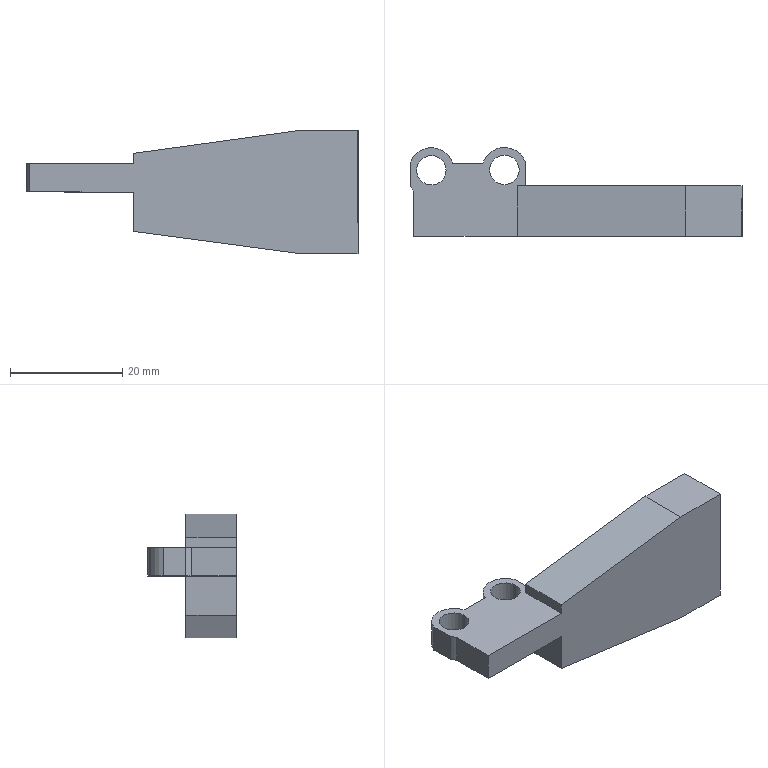Part | SolidWorks | features ICE 22, Fillet 4, Attribute 1, Extrusion 1, RevCut 1 | 1 solid | 22 faces | box 59.063 x 15.813 x 22 mm | volume 7989 mm3 | plane 15 | cylinder 7 | commonest cylinder face diameters 5.25 x4 8 x3
STEP:
#1=CARTESIAN_POINT('',(-7.896,-1.249,0.));
#2=VERTEX_POINT('',#1);
#3=CARTESIAN_POINT('',(-2.646,-1.249,0.));
#4=VERTEX_POINT('',#3);
#5=CARTESIAN_POINT('',(-5.271,-1.249,0.));
#6=DIRECTION('',(0.,0.,1.));
#7=DIRECTION('',(1.,0.,0.));
#8=AXIS2_PLACEMENT_3D('',#5,#6,#7);
#9=CIRCLE('',#8,2.625);
#10=EDGE_CURVE('',#2,#4,#9,.T.);
#11=ORIENTED_EDGE('',*,*,#10,.F.);
#12=CARTESIAN_POINT('',(-7.896,-1.249,5.));
#13=VERTEX_POINT('',#12);
#14=CARTESIAN_POINT('',(-7.896,-1.249,0.));
#15=DIRECTION('',(0.,0.,1.));
#16=VECTOR('',#15,1000.);
#17=LINE('',#14,#16);
#18=EDGE_CURVE('',#2,#13,#17,.T.);
#19=ORIENTED_EDGE('',*,*,#18,.T.);
#20=CARTESIAN_POINT('',(-2.646,-1.249,5.));
#21=VERTEX_POINT('',#20);
#22=CARTESIAN_POINT('',(-5.271,-1.249,5.));
#23=DIRECTION('',(0.,0.,1.));
#24=DIRECTION('',(1.,0.,0.));
#25=AXIS2_PLACEMENT_3D('',#22,#23,#24);
#26=CIRCLE('',#25,2.625);
#27=EDGE_CURVE('',#13,#21,#26,.T.);
#28=ORIENTED_EDGE('',*,*,#27,.T.);
#29=CARTESIAN_POINT('',(-2.646,-1.249,0.));
#30=DIRECTION('',(0.,0.,1.));
#31=VECTOR('',#30,1000.);
#32=LINE('',#29,#31);
#33=EDGE_CURVE('',#4,#21,#32,.T.);
#34=ORIENTED_EDGE('',*,*,#33,.F.);
#35=EDGE_LOOP('',(#11,#19,#28,#34));
#36=FACE_OUTER_BOUND('',#35,.T.);
#37=CARTESIAN_POINT('',(-5.271,-1.249,0.));
#38=DIRECTION('',(0.,0.,1.));
#39=DIRECTION('',(1.,0.,0.));
#40=AXIS2_PLACEMENT_3D('',#37,#38,#39);
#41=CYLINDRICAL_SURFACE('',#40,2.625);
#42=ADVANCED_FACE('',(#36),#41,.F.);
#43=CARTESIAN_POINT('',(5.104,-1.187,0.));
#44=VERTEX_POINT('',#43);
#45=CARTESIAN_POINT('',(10.354,-1.187,0.));
#46=VERTEX_POINT('',#45);
#47=CARTESIAN_POINT('',(7.729,-1.187,0.));
#48=DIRECTION('',(0.,0.,1.));
#49=DIRECTION('',(1.,0.,0.));
#50=AXIS2_PLACEMENT_3D('',#47,#48,#49);
#51=CIRCLE('',#50,2.625);
#52=EDGE_CURVE('',#44,#46,#51,.T.);
#53=ORIENTED_EDGE('',*,*,#52,.F.);
#54=CARTESIAN_POINT('',(5.104,-1.187,5.));
#55=VERTEX_POINT('',#54);
#56=CARTESIAN_POINT('',(5.104,-1.187,0.));
#57=DIRECTION('',(0.,0.,1.));
#58=VECTOR('',#57,1000.);
#59=LINE('',#56,#58);
#60=EDGE_CURVE('',#44,#55,#59,.T.);
#61=ORIENTED_EDGE('',*,*,#60,.T.);
#62=CARTESIAN_POINT('',(10.354,-1.187,5.));
#63=VERTEX_POINT('',#62);
#64=CARTESIAN_POINT('',(7.729,-1.187,5.));
#65=DIRECTION('',(0.,0.,1.));
#66=DIRECTION('',(1.,0.,0.));
#67=AXIS2_PLACEMENT_3D('',#64,#65,#66);
#68=CIRCLE('',#67,2.625);
#69=EDGE_CURVE('',#55,#63,#68,.T.);
#70=ORIENTED_EDGE('',*,*,#69,.T.);
#71=CARTESIAN_POINT('',(10.354,-1.187,0.));
#72=DIRECTION('',(0.,0.,1.));
#73=VECTOR('',#72,1000.);
#74=LINE('',#71,#73);
#75=EDGE_CURVE('',#46,#63,#74,.T.);
#76=ORIENTED_EDGE('',*,*,#75,.F.);
#77=EDGE_LOOP('',(#53,#61,#70,#76));
#78=FACE_OUTER_BOUND('',#77,.T.);
#79=CARTESIAN_POINT('',(7.729,-1.187,0.));
#80=DIRECTION('',(0.,0.,1.));
#81=DIRECTION('',(1.,0.,0.));
#82=AXIS2_PLACEMENT_3D('',#79,#80,#81);
#83=CYLINDRICAL_SURFACE('',#82,2.625);
#84=ADVANCED_FACE('',(#78),#83,.F.);
#85=CARTESIAN_POINT('',(-5.271,-1.249,0.));
#86=DIRECTION('',(0.,0.,1.));
#87=DIRECTION('',(1.,0.,0.));
#88=AXIS2_PLACEMENT_3D('',#85,#86,#87);
#89=CIRCLE('',#88,2.625);
#90=EDGE_CURVE('',#4,#2,#89,.T.);
#91=ORIENTED_EDGE('',*,*,#90,.T.);
#92=ORIENTED_EDGE('',*,*,#10,.T.);
#93=EDGE_LOOP('',(#91,#92));
#94=FACE_BOUND('',#93,.T.);
#95=CARTESIAN_POINT('',(7.729,-1.187,0.));
#96=DIRECTION('',(0.,0.,1.));
#97=DIRECTION('',(1.,0.,0.));
#98=AXIS2_PLACEMENT_3D('',#95,#96,#97);
#99=CIRCLE('',#98,2.625);
#100=EDGE_CURVE('',#46,#44,#99,.T.);
#101=ORIENTED_EDGE('',*,*,#100,.T.);
#102=ORIENTED_EDGE('',*,*,#52,.T.);
#103=EDGE_LOOP('',(#101,#102));
#104=FACE_BOUND('',#103,.T.);
#105=CARTESIAN_POINT('',(10.,-13.,0.));
#106=VERTEX_POINT('',#105);
#107=CARTESIAN_POINT('',(10.,-4.016,0.));
#108=VERTEX_POINT('',#107);
#109=CARTESIAN_POINT('',(10.,-54.478,0.));
#110=DIRECTION('',(0.,1.,0.));
#111=VECTOR('',#110,1000.);
#112=LINE('',#109,#111);
#113=EDGE_CURVE('',#106,#108,#112,.T.);
#114=ORIENTED_EDGE('',*,*,#113,.F.);
#115=CARTESIAN_POINT('',(-8.393,-13.,0.));
#116=VERTEX_POINT('',#115);
#117=CARTESIAN_POINT('',(-8.393,-13.,0.));
#118=DIRECTION('',(1.,0.,0.));
#119=VECTOR('',#118,1000.);
#120=LINE('',#117,#119);
#121=EDGE_CURVE('',#116,#106,#120,.T.);
#122=ORIENTED_EDGE('',*,*,#121,.F.);
#123=CARTESIAN_POINT('',(-8.393,-5.,0.));
#124=VERTEX_POINT('',#123);
#125=CARTESIAN_POINT('',(-8.393,-13.,0.));
#126=DIRECTION('',(0.,1.,0.));
#127=VECTOR('',#126,1000.);
#128=LINE('',#125,#127);
#129=EDGE_CURVE('',#116,#124,#128,.T.);
#130=ORIENTED_EDGE('',*,*,#129,.T.);
#131=CARTESIAN_POINT('',(-8.991,-3.97,0.));
#132=VERTEX_POINT('',#131);
#133=CARTESIAN_POINT('',(-5.271,-2.499,0.));
#134=DIRECTION('',(0.,0.,-1.));
#135=DIRECTION('',(-1.,0.,0.));
#136=AXIS2_PLACEMENT_3D('',#133,#134,#135);
#137=CIRCLE('',#136,4.);
#138=EDGE_CURVE('',#124,#132,#137,.T.);
#139=ORIENTED_EDGE('',*,*,#138,.T.);
#140=CARTESIAN_POINT('',(-9.071,0.,0.));
#141=VERTEX_POINT('',#140);
#142=CARTESIAN_POINT('',(-9.071,0.,0.));
#143=DIRECTION('',(0.02016,-0.9998,0.));
#144=VECTOR('',#143,1000.);
#145=LINE('',#142,#144);
#146=EDGE_CURVE('',#141,#132,#145,.T.);
#147=ORIENTED_EDGE('',*,*,#146,.F.);
#148=CARTESIAN_POINT('',(-1.471,0.,0.));
#149=VERTEX_POINT('',#148);
#150=CARTESIAN_POINT('',(-5.271,-1.249,0.));
#151=DIRECTION('',(0.,0.,-1.));
#152=DIRECTION('',(-1.,0.,0.));
#153=AXIS2_PLACEMENT_3D('',#150,#151,#152);
#154=CIRCLE('',#153,4.);
#155=EDGE_CURVE('',#141,#149,#154,.T.);
#156=ORIENTED_EDGE('',*,*,#155,.T.);
#157=CARTESIAN_POINT('',(3.909,0.,0.));
#158=VERTEX_POINT('',#157);
#159=CARTESIAN_POINT('',(0.,0.,0.));
#160=DIRECTION('',(1.,0.,0.));
#161=VECTOR('',#160,1000.);
#162=LINE('',#159,#161);
#163=EDGE_CURVE('',#149,#158,#162,.T.);
#164=ORIENTED_EDGE('',*,*,#163,.T.);
#165=CARTESIAN_POINT('',(11.505,0.1314,0.));
#166=VERTEX_POINT('',#165);
#167=CARTESIAN_POINT('',(7.729,-1.187,0.));
#168=DIRECTION('',(0.,0.,-1.));
#169=DIRECTION('',(-1.,0.,0.));
#170=AXIS2_PLACEMENT_3D('',#167,#168,#169);
#171=CIRCLE('',#170,4.);
#172=EDGE_CURVE('',#158,#166,#171,.T.);
#173=ORIENTED_EDGE('',*,*,#172,.T.);
#174=CARTESIAN_POINT('',(11.505,-4.016,0.));
#175=VERTEX_POINT('',#174);
#176=CARTESIAN_POINT('',(11.505,-2.579,0.));
#177=DIRECTION('',(0.,1.,0.));
#178=VECTOR('',#177,1000.);
#179=LINE('',#176,#178);
#180=EDGE_CURVE('',#175,#166,#179,.T.);
#181=ORIENTED_EDGE('',*,*,#180,.F.);
#182=CARTESIAN_POINT('',(49.993,-4.016,0.));
#183=DIRECTION('',(1.,0.,0.));
#184=VECTOR('',#183,1000.);
#185=LINE('',#182,#184);
#186=EDGE_CURVE('',#108,#175,#185,.T.);
#187=ORIENTED_EDGE('',*,*,#186,.F.);
#188=EDGE_LOOP('',(#114,#122,#130,#139,#147,#156,#164,#173,#181,#187));
#189=FACE_OUTER_BOUND('',#188,.T.);
#190=CARTESIAN_POINT('',(0.,0.,0.));
#191=DIRECTION('',(0.,0.,1.));
#192=DIRECTION('',(1.,0.,0.));
#193=AXIS2_PLACEMENT_3D('',#190,#191,#192);
#194=PLANE('',#193);
#195=ADVANCED_FACE('',(#94,#104,#189),#194,.F.);
#196=CARTESIAN_POINT('',(11.505,-4.016,5.));
#197=VERTEX_POINT('',#196);
#198=CARTESIAN_POINT('',(10.,-4.016,5.));
#199=VERTEX_POINT('',#198);
#200=CARTESIAN_POINT('',(10.,-4.016,5.));
#201=DIRECTION('',(-1.,0.,0.));
#202=VECTOR('',#201,1000.);
#203=LINE('',#200,#202);
#204=EDGE_CURVE('',#197,#199,#203,.T.);
#205=ORIENTED_EDGE('',*,*,#204,.F.);
#206=CARTESIAN_POINT('',(11.505,0.1314,5.));
#207=VERTEX_POINT('',#206);
#208=CARTESIAN_POINT('',(11.505,-2.579,5.));
#209=DIRECTION('',(0.,1.,0.));
#210=VECTOR('',#209,1000.);
#211=LINE('',#208,#210);
#212=EDGE_CURVE('',#197,#207,#211,.T.);
#213=ORIENTED_EDGE('',*,*,#212,.T.);
#214=CARTESIAN_POINT('',(3.909,0.,5.));
#215=VERTEX_POINT('',#214);
#216=CARTESIAN_POINT('',(7.729,-1.187,5.));
#217=DIRECTION('',(0.,0.,-1.));
#218=DIRECTION('',(-1.,0.,0.));
#219=AXIS2_PLACEMENT_3D('',#216,#217,#218);
#220=CIRCLE('',#219,4.);
#221=EDGE_CURVE('',#215,#207,#220,.T.);
#222=ORIENTED_EDGE('',*,*,#221,.F.);
#223=CARTESIAN_POINT('',(-1.471,0.,5.));
#224=VERTEX_POINT('',#223);
#225=CARTESIAN_POINT('',(0.,0.,5.));
#226=DIRECTION('',(-1.,0.,0.));
#227=VECTOR('',#226,1000.);
#228=LINE('',#225,#227);
#229=EDGE_CURVE('',#215,#224,#228,.T.);
#230=ORIENTED_EDGE('',*,*,#229,.T.);
#231=CARTESIAN_POINT('',(-9.071,0.,5.));
#232=VERTEX_POINT('',#231);
#233=CARTESIAN_POINT('',(-5.271,-1.249,5.));
#234=DIRECTION('',(0.,0.,-1.));
#235=DIRECTION('',(-1.,0.,0.));
#236=AXIS2_PLACEMENT_3D('',#233,#234,#235);
#237=CIRCLE('',#236,4.);
#238=EDGE_CURVE('',#232,#224,#237,.T.);
#239=ORIENTED_EDGE('',*,*,#238,.F.);
#240=CARTESIAN_POINT('',(-8.991,-3.97,5.));
#241=VERTEX_POINT('',#240);
#242=CARTESIAN_POINT('',(-9.071,0.,5.));
#243=DIRECTION('',(0.02016,-0.9998,0.));
#244=VECTOR('',#243,1000.);
#245=LINE('',#242,#244);
#246=EDGE_CURVE('',#232,#241,#245,.T.);
#247=ORIENTED_EDGE('',*,*,#246,.T.);
#248=CARTESIAN_POINT('',(-8.393,-5.,5.));
#249=VERTEX_POINT('',#248);
#250=CARTESIAN_POINT('',(-5.271,-2.499,5.));
#251=DIRECTION('',(0.,0.,-1.));
#252=DIRECTION('',(-1.,0.,0.));
#253=AXIS2_PLACEMENT_3D('',#250,#251,#252);
#254=CIRCLE('',#253,4.);
#255=EDGE_CURVE('',#249,#241,#254,.T.);
#256=ORIENTED_EDGE('',*,*,#255,.F.);
#257=CARTESIAN_POINT('',(-8.393,-13.,5.));
#258=VERTEX_POINT('',#257);
#259=CARTESIAN_POINT('',(-8.393,-13.,5.));
#260=DIRECTION('',(0.,1.,0.));
#261=VECTOR('',#260,1000.);
#262=LINE('',#259,#261);
#263=EDGE_CURVE('',#258,#249,#262,.T.);
#264=ORIENTED_EDGE('',*,*,#263,.F.);
#265=CARTESIAN_POINT('',(10.,-13.,5.));
#266=VERTEX_POINT('',#265);
#267=CARTESIAN_POINT('',(10.,-13.,5.));
#268=DIRECTION('',(-1.,0.,0.));
#269=VECTOR('',#268,1000.);
#270=LINE('',#267,#269);
#271=EDGE_CURVE('',#266,#258,#270,.T.);
#272=ORIENTED_EDGE('',*,*,#271,.F.);
#273=CARTESIAN_POINT('',(10.,-20.,5.));
#274=DIRECTION('',(0.,1.,0.));
#275=VECTOR('',#274,1000.);
#276=LINE('',#273,#275);
#277=EDGE_CURVE('',#266,#199,#276,.T.);
#278=ORIENTED_EDGE('',*,*,#277,.T.);
#279=EDGE_LOOP('',(#205,#213,#222,#230,#239,#247,#256,#264,#272,#278));
#280=FACE_OUTER_BOUND('',#279,.T.);
#281=CARTESIAN_POINT('',(7.729,-1.187,5.));
#282=DIRECTION('',(0.,0.,1.));
#283=DIRECTION('',(1.,0.,0.));
#284=AXIS2_PLACEMENT_3D('',#281,#282,#283);
#285=CIRCLE('',#284,2.625);
#286=EDGE_CURVE('',#63,#55,#285,.T.);
#287=ORIENTED_EDGE('',*,*,#286,.F.);
#288=ORIENTED_EDGE('',*,*,#69,.F.);
#289=EDGE_LOOP('',(#287,#288));
#290=FACE_BOUND('',#289,.T.);
#291=CARTESIAN_POINT('',(-5.271,-1.249,5.));
#292=DIRECTION('',(0.,0.,1.));
#293=DIRECTION('',(1.,0.,0.));
#294=AXIS2_PLACEMENT_3D('',#291,#292,#293);
#295=CIRCLE('',#294,2.625);
#296=EDGE_CURVE('',#21,#13,#295,.T.);
#297=ORIENTED_EDGE('',*,*,#296,.F.);
#298=ORIENTED_EDGE('',*,*,#27,.F.);
#299=EDGE_LOOP('',(#297,#298));
#300=FACE_BOUND('',#299,.T.);
#301=CARTESIAN_POINT('',(0.,-20.,5.));
#302=DIRECTION('',(0.,0.,-1.));
#303=DIRECTION('',(-1.,0.,0.));
#304=AXIS2_PLACEMENT_3D('',#301,#302,#303);
#305=PLANE('',#304);
#306=ADVANCED_FACE('',(#280,#290,#300),#305,.F.);
#307=CARTESIAN_POINT('',(10.,-13.,6.875));
#308=VERTEX_POINT('',#307);
#309=CARTESIAN_POINT('',(10.,-13.,8.751));
#310=DIRECTION('',(0.,0.,-1.));
#311=VECTOR('',#310,1000.);
#312=LINE('',#309,#311);
#313=EDGE_CURVE('',#308,#266,#312,.T.);
#314=ORIENTED_EDGE('',*,*,#313,.F.);
#315=CARTESIAN_POINT('',(10.,-4.016,6.875));
#316=VERTEX_POINT('',#315);
#317=CARTESIAN_POINT('',(10.,-3.,6.875));
#318=DIRECTION('',(0.,-1.,0.));
#319=VECTOR('',#318,1000.);
#320=LINE('',#317,#319);
#321=EDGE_CURVE('',#316,#308,#320,.T.);
#322=ORIENTED_EDGE('',*,*,#321,.F.);
#323=CARTESIAN_POINT('',(10.,-4.016,8.751));
#324=DIRECTION('',(0.,0.,1.));
#325=VECTOR('',#324,1000.);
#326=LINE('',#323,#325);
#327=EDGE_CURVE('',#199,#316,#326,.T.);
#328=ORIENTED_EDGE('',*,*,#327,.F.);
#329=ORIENTED_EDGE('',*,*,#277,.F.);
#330=EDGE_LOOP('',(#314,#322,#328,#329));
#331=FACE_OUTER_BOUND('',#330,.T.);
#332=CARTESIAN_POINT('',(10.,-20.,5.));
#333=DIRECTION('',(1.,0.,0.));
#334=DIRECTION('',(0.,0.,-1.));
#335=AXIS2_PLACEMENT_3D('',#332,#333,#334);
#336=PLANE('',#335);
#337=ADVANCED_FACE('',(#331),#336,.F.);
#338=CARTESIAN_POINT('',(-1.471,0.,5.));
#339=DIRECTION('',(0.,0.,-1.));
#340=VECTOR('',#339,1000.);
#341=LINE('',#338,#340);
#342=EDGE_CURVE('',#224,#149,#341,.T.);
#343=ORIENTED_EDGE('',*,*,#342,.F.);
#344=ORIENTED_EDGE('',*,*,#229,.F.);
#345=CARTESIAN_POINT('',(3.909,0.,5.));
#346=DIRECTION('',(0.,0.,1.));
#347=VECTOR('',#346,1000.);
#348=LINE('',#345,#347);
#349=EDGE_CURVE('',#158,#215,#348,.T.);
#350=ORIENTED_EDGE('',*,*,#349,.F.);
#351=ORIENTED_EDGE('',*,*,#163,.F.);
#352=EDGE_LOOP('',(#343,#344,#350,#351));
#353=FACE_OUTER_BOUND('',#352,.T.);
#354=CARTESIAN_POINT('',(0.,0.,20.));
#355=DIRECTION('',(0.,1.,0.));
#356=DIRECTION('',(0.,0.,1.));
#357=AXIS2_PLACEMENT_3D('',#354,#355,#356);
#358=PLANE('',#357);
#359=ADVANCED_FACE('',(#353),#358,.T.);
#360=CARTESIAN_POINT('',(39.993,-4.016,11.));
#361=VERTEX_POINT('',#360);
#362=CARTESIAN_POINT('',(51.022,-4.016,12.517));
#363=DIRECTION('',(0.9907,0.,0.1362));
#364=VECTOR('',#363,1000.);
#365=LINE('',#362,#364);
#366=EDGE_CURVE('',#316,#361,#365,.T.);
#367=ORIENTED_EDGE('',*,*,#366,.T.);
#368=CARTESIAN_POINT('',(49.993,-4.016,11.));
#369=VERTEX_POINT('',#368);
#370=CARTESIAN_POINT('',(49.993,-4.016,11.));
#371=DIRECTION('',(1.,0.,0.));
#372=VECTOR('',#371,1000.);
#373=LINE('',#370,#372);
#374=EDGE_CURVE('',#361,#369,#373,.T.);
#375=ORIENTED_EDGE('',*,*,#374,.T.);
#376=CARTESIAN_POINT('',(49.993,-4.016,-11.));
#377=VERTEX_POINT('',#376);
#378=CARTESIAN_POINT('',(49.993,-4.016,20.));
#379=DIRECTION('',(0.,0.,1.));
#380=VECTOR('',#379,1000.);
#381=LINE('',#378,#380);
#382=EDGE_CURVE('',#377,#369,#381,.T.);
#383=ORIENTED_EDGE('',*,*,#382,.F.);
#384=CARTESIAN_POINT('',(39.993,-4.016,-11.));
#385=VERTEX_POINT('',#384);
#386=CARTESIAN_POINT('',(49.993,-4.016,-11.));
#387=DIRECTION('',(-1.,0.,0.));
#388=VECTOR('',#387,1000.);
#389=LINE('',#386,#388);
#390=EDGE_CURVE('',#377,#385,#389,.T.);
#391=ORIENTED_EDGE('',*,*,#390,.T.);
#392=CARTESIAN_POINT('',(10.,-4.016,-7.));
#393=VERTEX_POINT('',#392);
#394=CARTESIAN_POINT('',(39.993,-4.016,-11.));
#395=DIRECTION('',(-0.9912,0.,0.1322));
#396=VECTOR('',#395,1000.);
#397=LINE('',#394,#396);
#398=EDGE_CURVE('',#385,#393,#397,.T.);
#399=ORIENTED_EDGE('',*,*,#398,.T.);
#400=CARTESIAN_POINT('',(10.,-4.016,-7.));
#401=DIRECTION('',(0.,0.,1.));
#402=VECTOR('',#401,1000.);
#403=LINE('',#400,#402);
#404=EDGE_CURVE('',#393,#108,#403,.T.);
#405=ORIENTED_EDGE('',*,*,#404,.T.);
#406=ORIENTED_EDGE('',*,*,#186,.T.);
#407=CARTESIAN_POINT('',(11.505,-4.016,20.));
#408=DIRECTION('',(0.,0.,1.));
#409=VECTOR('',#408,1000.);
#410=LINE('',#407,#409);
#411=EDGE_CURVE('',#175,#197,#410,.T.);
#412=ORIENTED_EDGE('',*,*,#411,.T.);
#413=ORIENTED_EDGE('',*,*,#204,.T.);
#414=ORIENTED_EDGE('',*,*,#327,.T.);
#415=EDGE_LOOP('',(#367,#375,#383,#391,#399,#405,#406,#412,#413,#414));
#416=FACE_OUTER_BOUND('',#415,.T.);
#417=CARTESIAN_POINT('',(49.993,-4.016,20.));
#418=DIRECTION('',(0.,-1.,0.));
#419=DIRECTION('',(0.,0.,-1.));
#420=AXIS2_PLACEMENT_3D('',#417,#418,#419);
#421=PLANE('',#420);
#422=ADVANCED_FACE('',(#416),#421,.F.);
#423=CARTESIAN_POINT('',(49.993,-13.,11.));
#424=VERTEX_POINT('',#423);
#425=CARTESIAN_POINT('',(49.993,-3.,11.));
#426=DIRECTION('',(0.,-1.,0.));
#427=VECTOR('',#426,1000.);
#428=LINE('',#425,#427);
#429=EDGE_CURVE('',#369,#424,#428,.T.);
#430=ORIENTED_EDGE('',*,*,#429,.T.);
#431=CARTESIAN_POINT('',(49.993,-13.,-11.));
#432=VERTEX_POINT('',#431);
#433=CARTESIAN_POINT('',(49.993,-13.,0.));
#434=DIRECTION('',(0.,0.,1.));
#435=VECTOR('',#434,1000.);
#436=LINE('',#433,#435);
#437=EDGE_CURVE('',#432,#424,#436,.T.);
#438=ORIENTED_EDGE('',*,*,#437,.F.);
#439=CARTESIAN_POINT('',(49.993,-54.478,-11.));
#440=DIRECTION('',(0.,1.,0.));
#441=VECTOR('',#440,1000.);
#442=LINE('',#439,#441);
#443=EDGE_CURVE('',#432,#377,#442,.T.);
#444=ORIENTED_EDGE('',*,*,#443,.T.);
#445=ORIENTED_EDGE('',*,*,#382,.T.);
#446=EDGE_LOOP('',(#430,#438,#444,#445));
#447=FACE_OUTER_BOUND('',#446,.T.);
#448=CARTESIAN_POINT('',(49.993,0.,0.));
#449=DIRECTION('',(1.,0.,0.));
#450=DIRECTION('',(0.,0.,-1.));
#451=AXIS2_PLACEMENT_3D('',#448,#449,#450);
#452=PLANE('',#451);
#453=ADVANCED_FACE('',(#447),#452,.T.);
#454=CARTESIAN_POINT('',(-8.991,-3.97,5.));
#455=DIRECTION('',(0.,0.,-1.));
#456=VECTOR('',#455,1000.);
#457=LINE('',#454,#456);
#458=EDGE_CURVE('',#241,#132,#457,.T.);
#459=ORIENTED_EDGE('',*,*,#458,.T.);
#460=ORIENTED_EDGE('',*,*,#138,.F.);
#461=CARTESIAN_POINT('',(-8.393,-5.,5.));
#462=DIRECTION('',(0.,0.,-1.));
#463=VECTOR('',#462,1000.);
#464=LINE('',#461,#463);
#465=EDGE_CURVE('',#249,#124,#464,.T.);
#466=ORIENTED_EDGE('',*,*,#465,.F.);
#467=ORIENTED_EDGE('',*,*,#255,.T.);
#468=EDGE_LOOP('',(#459,#460,#466,#467));
#469=FACE_OUTER_BOUND('',#468,.T.);
#470=CARTESIAN_POINT('',(-5.271,-2.499,5.));
#471=DIRECTION('',(0.,0.,-1.));
#472=DIRECTION('',(-1.,0.,0.));
#473=AXIS2_PLACEMENT_3D('',#470,#471,#472);
#474=CYLINDRICAL_SURFACE('',#473,4.);
#475=ADVANCED_FACE('',(#469),#474,.T.);
#476=CARTESIAN_POINT('',(11.505,0.1314,5.));
#477=DIRECTION('',(0.,0.,1.));
#478=VECTOR('',#477,1000.);
#479=LINE('',#476,#478);
#480=EDGE_CURVE('',#166,#207,#479,.T.);
#481=ORIENTED_EDGE('',*,*,#480,.F.);
#482=ORIENTED_EDGE('',*,*,#172,.F.);
#483=ORIENTED_EDGE('',*,*,#349,.T.);
#484=ORIENTED_EDGE('',*,*,#221,.T.);
#485=EDGE_LOOP('',(#481,#482,#483,#484));
#486=FACE_OUTER_BOUND('',#485,.T.);
#487=CARTESIAN_POINT('',(7.729,-1.187,5.));
#488=DIRECTION('',(0.,0.,-1.));
#489=DIRECTION('',(-1.,0.,0.));
#490=AXIS2_PLACEMENT_3D('',#487,#488,#489);
#491=CYLINDRICAL_SURFACE('',#490,4.);
#492=ADVANCED_FACE('',(#486),#491,.T.);
#493=CARTESIAN_POINT('',(-9.071,0.,5.));
#494=DIRECTION('',(0.,0.,-1.));
#495=VECTOR('',#494,1000.);
#496=LINE('',#493,#495);
#497=EDGE_CURVE('',#232,#141,#496,.T.);
#498=ORIENTED_EDGE('',*,*,#497,.F.);
#499=ORIENTED_EDGE('',*,*,#238,.T.);
#500=ORIENTED_EDGE('',*,*,#342,.T.);
#501=ORIENTED_EDGE('',*,*,#155,.F.);
#502=EDGE_LOOP('',(#498,#499,#500,#501));
#503=FACE_OUTER_BOUND('',#502,.T.);
#504=CARTESIAN_POINT('',(-5.271,-1.249,5.));
#505=DIRECTION('',(0.,0.,-1.));
#506=DIRECTION('',(-1.,0.,0.));
#507=AXIS2_PLACEMENT_3D('',#504,#505,#506);
#508=CYLINDRICAL_SURFACE('',#507,4.);
#509=ADVANCED_FACE('',(#503),#508,.T.);
#510=ORIENTED_EDGE('',*,*,#146,.T.);
#511=ORIENTED_EDGE('',*,*,#458,.F.);
#512=ORIENTED_EDGE('',*,*,#246,.F.);
#513=ORIENTED_EDGE('',*,*,#497,.T.);
#514=EDGE_LOOP('',(#510,#511,#512,#513));
#515=FACE_OUTER_BOUND('',#514,.T.);
#516=CARTESIAN_POINT('',(-9.071,0.,5.));
#517=DIRECTION('',(0.9998,0.02016,0.));
#518=DIRECTION('',(-0.02016,0.9998,0.));
#519=AXIS2_PLACEMENT_3D('',#516,#517,#518);
#520=PLANE('',#519);
#521=ADVANCED_FACE('',(#515),#520,.F.);
#522=ORIENTED_EDGE('',*,*,#212,.F.);
#523=ORIENTED_EDGE('',*,*,#411,.F.);
#524=ORIENTED_EDGE('',*,*,#180,.T.);
#525=ORIENTED_EDGE('',*,*,#480,.T.);
#526=EDGE_LOOP('',(#522,#523,#524,#525));
#527=FACE_OUTER_BOUND('',#526,.T.);
#528=CARTESIAN_POINT('',(11.505,-2.579,5.));
#529=DIRECTION('',(-1.,0.,0.));
#530=DIRECTION('',(0.,0.,1.));
#531=AXIS2_PLACEMENT_3D('',#528,#529,#530);
#532=PLANE('',#531);
#533=ADVANCED_FACE('',(#527),#532,.F.);
#534=ORIENTED_EDGE('',*,*,#60,.F.);
#535=ORIENTED_EDGE('',*,*,#100,.F.);
#536=ORIENTED_EDGE('',*,*,#75,.T.);
#537=ORIENTED_EDGE('',*,*,#286,.T.);
#538=EDGE_LOOP('',(#534,#535,#536,#537));
#539=FACE_OUTER_BOUND('',#538,.T.);
#540=CARTESIAN_POINT('',(7.729,-1.187,0.));
#541=DIRECTION('',(0.,0.,1.));
#542=DIRECTION('',(1.,0.,0.));
#543=AXIS2_PLACEMENT_3D('',#540,#541,#542);
#544=CYLINDRICAL_SURFACE('',#543,2.625);
#545=ADVANCED_FACE('',(#539),#544,.F.);
#546=ORIENTED_EDGE('',*,*,#18,.F.);
#547=ORIENTED_EDGE('',*,*,#90,.F.);
#548=ORIENTED_EDGE('',*,*,#33,.T.);
#549=ORIENTED_EDGE('',*,*,#296,.T.);
#550=EDGE_LOOP('',(#546,#547,#548,#549));
#551=FACE_OUTER_BOUND('',#550,.T.);
#552=CARTESIAN_POINT('',(-5.271,-1.249,0.));
#553=DIRECTION('',(0.,0.,1.));
#554=DIRECTION('',(1.,0.,0.));
#555=AXIS2_PLACEMENT_3D('',#552,#553,#554);
#556=CYLINDRICAL_SURFACE('',#555,2.625);
#557=ADVANCED_FACE('',(#551),#556,.F.);
#558=ORIENTED_EDGE('',*,*,#465,.T.);
#559=ORIENTED_EDGE('',*,*,#129,.F.);
#560=CARTESIAN_POINT('',(-8.393,-13.,5.));
#561=DIRECTION('',(0.,0.,-1.));
#562=VECTOR('',#561,1000.);
#563=LINE('',#560,#562);
#564=EDGE_CURVE('',#258,#116,#563,.T.);
#565=ORIENTED_EDGE('',*,*,#564,.F.);
#566=ORIENTED_EDGE('',*,*,#263,.T.);
#567=EDGE_LOOP('',(#558,#559,#565,#566));
#568=FACE_OUTER_BOUND('',#567,.T.);
#569=CARTESIAN_POINT('',(-8.393,-13.,5.));
#570=DIRECTION('',(1.,0.,0.));
#571=DIRECTION('',(0.,0.,-1.));
#572=AXIS2_PLACEMENT_3D('',#569,#570,#571);
#573=PLANE('',#572);
#574=ADVANCED_FACE('',(#568),#573,.F.);
#575=CARTESIAN_POINT('',(39.993,-13.,11.));
#576=VERTEX_POINT('',#575);
#577=CARTESIAN_POINT('',(39.993,-13.,11.));
#578=DIRECTION('',(1.,0.,0.));
#579=VECTOR('',#578,1000.);
#580=LINE('',#577,#579);
#581=EDGE_CURVE('',#576,#424,#580,.T.);
#582=ORIENTED_EDGE('',*,*,#581,.F.);
#583=CARTESIAN_POINT('',(10.,-13.,6.875));
#584=DIRECTION('',(0.9907,0.,0.1362));
#585=VECTOR('',#584,1000.);
#586=LINE('',#583,#585);
#587=EDGE_CURVE('',#308,#576,#586,.T.);
#588=ORIENTED_EDGE('',*,*,#587,.F.);
#589=ORIENTED_EDGE('',*,*,#313,.T.);
#590=ORIENTED_EDGE('',*,*,#271,.T.);
#591=ORIENTED_EDGE('',*,*,#564,.T.);
#592=ORIENTED_EDGE('',*,*,#121,.T.);
#593=CARTESIAN_POINT('',(10.,-13.,-7.));
#594=VERTEX_POINT('',#593);
#595=CARTESIAN_POINT('',(10.,-13.,-7.));
#596=DIRECTION('',(0.,0.,1.));
#597=VECTOR('',#596,1000.);
#598=LINE('',#595,#597);
#599=EDGE_CURVE('',#594,#106,#598,.T.);
#600=ORIENTED_EDGE('',*,*,#599,.F.);
#601=CARTESIAN_POINT('',(39.993,-13.,-11.));
#602=VERTEX_POINT('',#601);
#603=CARTESIAN_POINT('',(39.993,-13.,-11.));
#604=DIRECTION('',(-0.9912,0.,0.1322));
#605=VECTOR('',#604,1000.);
#606=LINE('',#603,#605);
#607=EDGE_CURVE('',#602,#594,#606,.T.);
#608=ORIENTED_EDGE('',*,*,#607,.F.);
#609=CARTESIAN_POINT('',(49.993,-13.,-11.));
#610=DIRECTION('',(-1.,0.,0.));
#611=VECTOR('',#610,1000.);
#612=LINE('',#609,#611);
#613=EDGE_CURVE('',#432,#602,#612,.T.);
#614=ORIENTED_EDGE('',*,*,#613,.F.);
#615=ORIENTED_EDGE('',*,*,#437,.T.);
#616=EDGE_LOOP('',(#582,#588,#589,#590,#591,#592,#600,#608,#614,#615));
#617=FACE_OUTER_BOUND('',#616,.T.);
#618=CARTESIAN_POINT('',(0.,-13.,0.));
#619=DIRECTION('',(0.,-1.,0.));
#620=DIRECTION('',(0.,0.,-1.));
#621=AXIS2_PLACEMENT_3D('',#618,#619,#620);
#622=PLANE('',#621);
#623=ADVANCED_FACE('',(#617),#622,.T.);
#624=CARTESIAN_POINT('',(39.993,-3.,11.));
#625=DIRECTION('',(0.,-1.,0.));
#626=VECTOR('',#625,1000.);
#627=LINE('',#624,#626);
#628=EDGE_CURVE('',#361,#576,#627,.T.);
#629=ORIENTED_EDGE('',*,*,#628,.T.);
#630=ORIENTED_EDGE('',*,*,#581,.T.);
#631=ORIENTED_EDGE('',*,*,#429,.F.);
#632=ORIENTED_EDGE('',*,*,#374,.F.);
#633=EDGE_LOOP('',(#629,#630,#631,#632));
#634=FACE_OUTER_BOUND('',#633,.T.);
#635=CARTESIAN_POINT('',(39.993,-3.,11.));
#636=DIRECTION('',(0.,0.,-1.));
#637=DIRECTION('',(-1.,0.,0.));
#638=AXIS2_PLACEMENT_3D('',#635,#636,#637);
#639=PLANE('',#638);
#640=ADVANCED_FACE('',(#634),#639,.F.);
#641=ORIENTED_EDGE('',*,*,#321,.T.);
#642=ORIENTED_EDGE('',*,*,#587,.T.);
#643=ORIENTED_EDGE('',*,*,#628,.F.);
#644=ORIENTED_EDGE('',*,*,#366,.F.);
#645=EDGE_LOOP('',(#641,#642,#643,#644));
#646=FACE_OUTER_BOUND('',#645,.T.);
#647=CARTESIAN_POINT('',(10.,-3.,6.875));
#648=DIRECTION('',(0.1362,0.,-0.9907));
#649=DIRECTION('',(-0.9907,0.,-0.1362));
#650=AXIS2_PLACEMENT_3D('',#647,#648,#649);
#651=PLANE('',#650);
#652=ADVANCED_FACE('',(#646),#651,.F.);
#653=ORIENTED_EDGE('',*,*,#443,.F.);
#654=ORIENTED_EDGE('',*,*,#613,.T.);
#655=CARTESIAN_POINT('',(39.993,-54.478,-11.));
#656=DIRECTION('',(0.,1.,0.));
#657=VECTOR('',#656,1000.);
#658=LINE('',#655,#657);
#659=EDGE_CURVE('',#602,#385,#658,.T.);
#660=ORIENTED_EDGE('',*,*,#659,.T.);
#661=ORIENTED_EDGE('',*,*,#390,.F.);
#662=EDGE_LOOP('',(#653,#654,#660,#661));
#663=FACE_OUTER_BOUND('',#662,.T.);
#664=CARTESIAN_POINT('',(49.993,-54.478,-11.));
#665=DIRECTION('',(0.,0.,-1.));
#666=DIRECTION('',(-1.,0.,0.));
#667=AXIS2_PLACEMENT_3D('',#664,#665,#666);
#668=PLANE('',#667);
#669=ADVANCED_FACE('',(#663),#668,.T.);
#670=ORIENTED_EDGE('',*,*,#659,.F.);
#671=ORIENTED_EDGE('',*,*,#607,.T.);
#672=CARTESIAN_POINT('',(10.,-54.478,-7.));
#673=DIRECTION('',(0.,1.,0.));
#674=VECTOR('',#673,1000.);
#675=LINE('',#672,#674);
#676=EDGE_CURVE('',#594,#393,#675,.T.);
#677=ORIENTED_EDGE('',*,*,#676,.T.);
#678=ORIENTED_EDGE('',*,*,#398,.F.);
#679=EDGE_LOOP('',(#670,#671,#677,#678));
#680=FACE_OUTER_BOUND('',#679,.T.);
#681=CARTESIAN_POINT('',(39.993,-54.478,-11.));
#682=DIRECTION('',(-0.1322,0.,-0.9912));
#683=DIRECTION('',(-0.9912,0.,0.1322));
#684=AXIS2_PLACEMENT_3D('',#681,#682,#683);
#685=PLANE('',#684);
#686=ADVANCED_FACE('',(#680),#685,.T.);
#687=ORIENTED_EDGE('',*,*,#676,.F.);
#688=ORIENTED_EDGE('',*,*,#599,.T.);
#689=ORIENTED_EDGE('',*,*,#113,.T.);
#690=ORIENTED_EDGE('',*,*,#404,.F.);
#691=EDGE_LOOP('',(#687,#688,#689,#690));
#692=FACE_OUTER_BOUND('',#691,.T.);
#693=CARTESIAN_POINT('',(10.,-54.478,-7.));
#694=DIRECTION('',(-1.,0.,0.));
#695=DIRECTION('',(0.,-1.,0.));
#696=AXIS2_PLACEMENT_3D('',#693,#694,#695);
#697=PLANE('',#696);
#698=ADVANCED_FACE('',(#692),#697,.T.);
#699=CLOSED_SHELL('',(#42,#84,#195,#306,#337,#359,#422,#453,#475,#492,#509,#521,#533,#545,#557,#574,#623,#640,#652,#669,#686,#698));
#700=MANIFOLD_SOLID_BREP('',#699);
#701=CARTESIAN_POINT('',(0.,0.,0.));
#702=DIRECTION('',(0.,0.,1.));
#703=DIRECTION('',(1.,0.,0.));
#704=AXIS2_PLACEMENT_3D('',#701,#702,#703);
#705=(LENGTH_UNIT()NAMED_UNIT(*)SI_UNIT(.MILLI.,.METRE.));
#706=UNCERTAINTY_MEASURE_WITH_UNIT(LENGTH_MEASURE(0.00001),#705,'','');
#707=(NAMED_UNIT(*)PLANE_ANGLE_UNIT()SI_UNIT($,.RADIAN.));
#708=(NAMED_UNIT(*)SI_UNIT($,.STERADIAN.)SOLID_ANGLE_UNIT());
#709=(GEOMETRIC_REPRESENTATION_CONTEXT(3)GLOBAL_UNCERTAINTY_ASSIGNED_CONTEXT((#706))GLOBAL_UNIT_ASSIGNED_CONTEXT((#705,#707,#708))REPRESENTATION_CONTEXT('',''));
#710=ADVANCED_BREP_SHAPE_REPRESENTATION('',(#700,#704),#709);